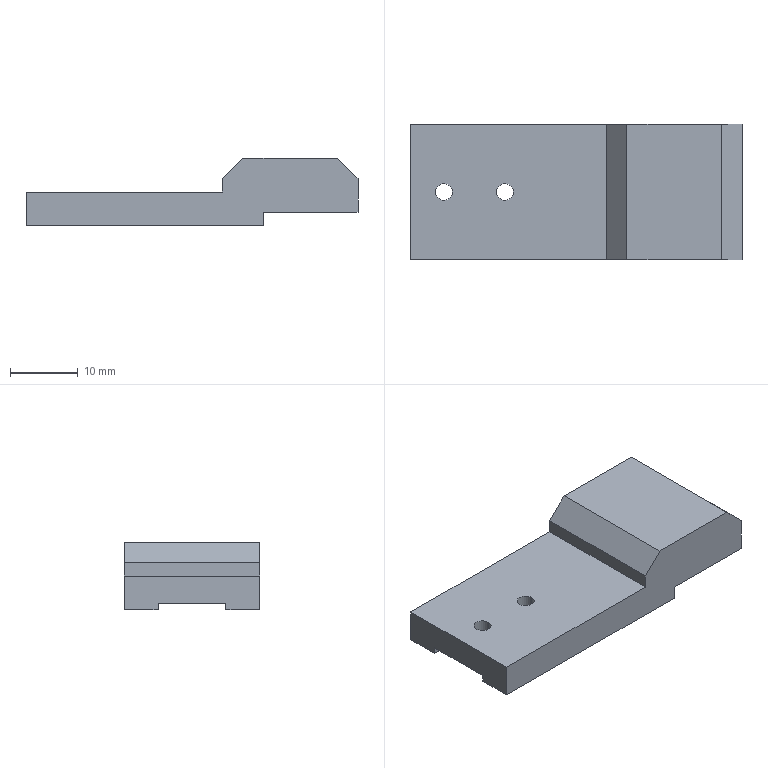Part | SolidWorks | features ICE 4, Chamfer 2, Extrusion 1, HoleWzd 1, MoveFace 1 | 1 solid | 20 faces | box 49 x 20 x 10 mm | volume 5771 mm3 | plane 16 | cylinder 4 | commonest cylinder face diameters 2.5 x4
STEP:
#1=CARTESIAN_POINT('',(-8.75,0.,1.));
#2=VERTEX_POINT('',#1);
#3=CARTESIAN_POINT('',(-11.25,0.,1.));
#4=VERTEX_POINT('',#3);
#5=CARTESIAN_POINT('',(-10.,0.,1.));
#6=DIRECTION('',(0.,0.,-1.));
#7=DIRECTION('',(-1.,0.,0.));
#8=AXIS2_PLACEMENT_3D('',#5,#6,#7);
#9=CIRCLE('',#8,1.25);
#10=EDGE_CURVE('',#2,#4,#9,.T.);
#11=ORIENTED_EDGE('',*,*,#10,.T.);
#12=CARTESIAN_POINT('',(-11.25,0.,5.));
#13=VERTEX_POINT('',#12);
#14=CARTESIAN_POINT('',(-11.25,0.,5.));
#15=DIRECTION('',(0.,0.,1.));
#16=VECTOR('',#15,1000.);
#17=LINE('',#14,#16);
#18=EDGE_CURVE('',#4,#13,#17,.T.);
#19=ORIENTED_EDGE('',*,*,#18,.T.);
#20=CARTESIAN_POINT('',(-8.75,0.,5.));
#21=VERTEX_POINT('',#20);
#22=CARTESIAN_POINT('',(-10.,0.,5.));
#23=DIRECTION('',(0.,0.,1.));
#24=DIRECTION('',(1.,0.,0.));
#25=AXIS2_PLACEMENT_3D('',#22,#23,#24);
#26=CIRCLE('',#25,1.25);
#27=EDGE_CURVE('',#13,#21,#26,.T.);
#28=ORIENTED_EDGE('',*,*,#27,.T.);
#29=CARTESIAN_POINT('',(-8.75,0.,5.));
#30=DIRECTION('',(0.,0.,1.));
#31=VECTOR('',#30,1000.);
#32=LINE('',#29,#31);
#33=EDGE_CURVE('',#2,#21,#32,.T.);
#34=ORIENTED_EDGE('',*,*,#33,.F.);
#35=EDGE_LOOP('',(#11,#19,#28,#34));
#36=FACE_OUTER_BOUND('',#35,.T.);
#37=CARTESIAN_POINT('',(-10.,0.,5.));
#38=DIRECTION('',(0.,0.,1.));
#39=DIRECTION('',(1.,0.,0.));
#40=AXIS2_PLACEMENT_3D('',#37,#38,#39);
#41=CYLINDRICAL_SURFACE('',#40,1.25);
#42=ADVANCED_FACE('',(#36),#41,.F.);
#43=CARTESIAN_POINT('',(0.25,0.,1.));
#44=VERTEX_POINT('',#43);
#45=CARTESIAN_POINT('',(-2.25,0.,1.));
#46=VERTEX_POINT('',#45);
#47=CARTESIAN_POINT('',(-1.,0.,1.));
#48=DIRECTION('',(0.,0.,-1.));
#49=DIRECTION('',(-1.,0.,0.));
#50=AXIS2_PLACEMENT_3D('',#47,#48,#49);
#51=CIRCLE('',#50,1.25);
#52=EDGE_CURVE('',#44,#46,#51,.T.);
#53=ORIENTED_EDGE('',*,*,#52,.T.);
#54=CARTESIAN_POINT('',(-2.25,0.,5.));
#55=VERTEX_POINT('',#54);
#56=CARTESIAN_POINT('',(-2.25,0.,5.));
#57=DIRECTION('',(0.,0.,1.));
#58=VECTOR('',#57,1000.);
#59=LINE('',#56,#58);
#60=EDGE_CURVE('',#46,#55,#59,.T.);
#61=ORIENTED_EDGE('',*,*,#60,.T.);
#62=CARTESIAN_POINT('',(0.25,0.,5.));
#63=VERTEX_POINT('',#62);
#64=CARTESIAN_POINT('',(-1.,0.,5.));
#65=DIRECTION('',(0.,0.,1.));
#66=DIRECTION('',(1.,0.,0.));
#67=AXIS2_PLACEMENT_3D('',#64,#65,#66);
#68=CIRCLE('',#67,1.25);
#69=EDGE_CURVE('',#55,#63,#68,.T.);
#70=ORIENTED_EDGE('',*,*,#69,.T.);
#71=CARTESIAN_POINT('',(0.25,0.,5.));
#72=DIRECTION('',(0.,0.,1.));
#73=VECTOR('',#72,1000.);
#74=LINE('',#71,#73);
#75=EDGE_CURVE('',#44,#63,#74,.T.);
#76=ORIENTED_EDGE('',*,*,#75,.F.);
#77=EDGE_LOOP('',(#53,#61,#70,#76));
#78=FACE_OUTER_BOUND('',#77,.T.);
#79=CARTESIAN_POINT('',(-1.,0.,5.));
#80=DIRECTION('',(0.,0.,1.));
#81=DIRECTION('',(1.,0.,0.));
#82=AXIS2_PLACEMENT_3D('',#79,#80,#81);
#83=CYLINDRICAL_SURFACE('',#82,1.25);
#84=ADVANCED_FACE('',(#78),#83,.F.);
#85=CARTESIAN_POINT('',(-15.,-5.,0.));
#86=VERTEX_POINT('',#85);
#87=CARTESIAN_POINT('',(-15.,-10.,0.));
#88=VERTEX_POINT('',#87);
#89=CARTESIAN_POINT('',(-15.,10.,0.));
#90=DIRECTION('',(0.,-1.,0.));
#91=VECTOR('',#90,1000.);
#92=LINE('',#89,#91);
#93=EDGE_CURVE('',#86,#88,#92,.T.);
#94=ORIENTED_EDGE('',*,*,#93,.F.);
#95=CARTESIAN_POINT('',(20.,-5.,0.));
#96=VERTEX_POINT('',#95);
#97=CARTESIAN_POINT('',(-15.,-5.,0.));
#98=DIRECTION('',(-1.,0.,0.));
#99=VECTOR('',#98,1000.);
#100=LINE('',#97,#99);
#101=EDGE_CURVE('',#96,#86,#100,.T.);
#102=ORIENTED_EDGE('',*,*,#101,.F.);
#103=CARTESIAN_POINT('',(20.,-10.,0.));
#104=VERTEX_POINT('',#103);
#105=CARTESIAN_POINT('',(20.,10.,0.));
#106=DIRECTION('',(0.,1.,0.));
#107=VECTOR('',#106,1000.);
#108=LINE('',#105,#107);
#109=EDGE_CURVE('',#104,#96,#108,.T.);
#110=ORIENTED_EDGE('',*,*,#109,.F.);
#111=CARTESIAN_POINT('',(-15.,-10.,0.));
#112=DIRECTION('',(1.,0.,0.));
#113=VECTOR('',#112,1000.);
#114=LINE('',#111,#113);
#115=EDGE_CURVE('',#88,#104,#114,.T.);
#116=ORIENTED_EDGE('',*,*,#115,.F.);
#117=EDGE_LOOP('',(#94,#102,#110,#116));
#118=FACE_OUTER_BOUND('',#117,.T.);
#119=CARTESIAN_POINT('',(0.,0.,0.));
#120=DIRECTION('',(0.,0.,1.));
#121=DIRECTION('',(1.,0.,0.));
#122=AXIS2_PLACEMENT_3D('',#119,#120,#121);
#123=PLANE('',#122);
#124=ADVANCED_FACE('',(#118),#123,.F.);
#125=CARTESIAN_POINT('',(31.,10.,10.));
#126=VERTEX_POINT('',#125);
#127=CARTESIAN_POINT('',(17.,10.,10.));
#128=VERTEX_POINT('',#127);
#129=CARTESIAN_POINT('',(14.,10.,10.));
#130=DIRECTION('',(-1.,0.,0.));
#131=VECTOR('',#130,1000.);
#132=LINE('',#129,#131);
#133=EDGE_CURVE('',#126,#128,#132,.T.);
#134=ORIENTED_EDGE('',*,*,#133,.F.);
#135=CARTESIAN_POINT('',(34.,10.,7.));
#136=VERTEX_POINT('',#135);
#137=CARTESIAN_POINT('',(31.,10.,10.));
#138=DIRECTION('',(0.7071,0.,-0.7071));
#139=VECTOR('',#138,1000.);
#140=LINE('',#137,#139);
#141=EDGE_CURVE('',#126,#136,#140,.T.);
#142=ORIENTED_EDGE('',*,*,#141,.T.);
#143=CARTESIAN_POINT('',(34.,10.,2.));
#144=VERTEX_POINT('',#143);
#145=CARTESIAN_POINT('',(34.,10.,10.));
#146=DIRECTION('',(0.,0.,-1.));
#147=VECTOR('',#146,1000.);
#148=LINE('',#145,#147);
#149=EDGE_CURVE('',#136,#144,#148,.T.);
#150=ORIENTED_EDGE('',*,*,#149,.T.);
#151=CARTESIAN_POINT('',(20.,10.,2.));
#152=VERTEX_POINT('',#151);
#153=CARTESIAN_POINT('',(14.,10.,2.));
#154=DIRECTION('',(-1.,0.,0.));
#155=VECTOR('',#154,1000.);
#156=LINE('',#153,#155);
#157=EDGE_CURVE('',#144,#152,#156,.T.);
#158=ORIENTED_EDGE('',*,*,#157,.T.);
#159=CARTESIAN_POINT('',(20.,10.,0.));
#160=VERTEX_POINT('',#159);
#161=CARTESIAN_POINT('',(20.,10.,0.));
#162=DIRECTION('',(0.,0.,1.));
#163=VECTOR('',#162,1000.);
#164=LINE('',#161,#163);
#165=EDGE_CURVE('',#160,#152,#164,.T.);
#166=ORIENTED_EDGE('',*,*,#165,.F.);
#167=CARTESIAN_POINT('',(-15.,10.,0.));
#168=VERTEX_POINT('',#167);
#169=CARTESIAN_POINT('',(-15.,10.,0.));
#170=DIRECTION('',(-1.,0.,0.));
#171=VECTOR('',#170,1000.);
#172=LINE('',#169,#171);
#173=EDGE_CURVE('',#160,#168,#172,.T.);
#174=ORIENTED_EDGE('',*,*,#173,.T.);
#175=CARTESIAN_POINT('',(-15.,10.,5.));
#176=VERTEX_POINT('',#175);
#177=CARTESIAN_POINT('',(-15.,10.,5.));
#178=DIRECTION('',(0.,0.,-1.));
#179=VECTOR('',#178,1000.);
#180=LINE('',#177,#179);
#181=EDGE_CURVE('',#176,#168,#180,.T.);
#182=ORIENTED_EDGE('',*,*,#181,.F.);
#183=CARTESIAN_POINT('',(14.,10.,5.));
#184=VERTEX_POINT('',#183);
#185=CARTESIAN_POINT('',(-15.,10.,5.));
#186=DIRECTION('',(-1.,0.,0.));
#187=VECTOR('',#186,1000.);
#188=LINE('',#185,#187);
#189=EDGE_CURVE('',#184,#176,#188,.T.);
#190=ORIENTED_EDGE('',*,*,#189,.F.);
#191=CARTESIAN_POINT('',(14.,10.,7.));
#192=VERTEX_POINT('',#191);
#193=CARTESIAN_POINT('',(14.,10.,10.));
#194=DIRECTION('',(0.,0.,-1.));
#195=VECTOR('',#194,1000.);
#196=LINE('',#193,#195);
#197=EDGE_CURVE('',#192,#184,#196,.T.);
#198=ORIENTED_EDGE('',*,*,#197,.F.);
#199=CARTESIAN_POINT('',(17.,10.,10.));
#200=DIRECTION('',(0.7071,0.,0.7071));
#201=VECTOR('',#200,1000.);
#202=LINE('',#199,#201);
#203=EDGE_CURVE('',#192,#128,#202,.T.);
#204=ORIENTED_EDGE('',*,*,#203,.T.);
#205=EDGE_LOOP('',(#134,#142,#150,#158,#166,#174,#182,#190,#198,#204));
#206=FACE_OUTER_BOUND('',#205,.T.);
#207=CARTESIAN_POINT('',(-15.,10.,5.));
#208=DIRECTION('',(0.,-1.,0.));
#209=DIRECTION('',(0.,0.,-1.));
#210=AXIS2_PLACEMENT_3D('',#207,#208,#209);
#211=PLANE('',#210);
#212=ADVANCED_FACE('',(#206),#211,.F.);
#213=CARTESIAN_POINT('',(-15.,-5.,1.));
#214=VERTEX_POINT('',#213);
#215=CARTESIAN_POINT('',(-15.,5.,1.));
#216=VERTEX_POINT('',#215);
#217=CARTESIAN_POINT('',(-15.,-5.,1.));
#218=DIRECTION('',(0.,1.,0.));
#219=VECTOR('',#218,1000.);
#220=LINE('',#217,#219);
#221=EDGE_CURVE('',#214,#216,#220,.T.);
#222=ORIENTED_EDGE('',*,*,#221,.F.);
#223=CARTESIAN_POINT('',(-15.,-5.,1.));
#224=DIRECTION('',(0.,0.,-1.));
#225=VECTOR('',#224,1000.);
#226=LINE('',#223,#225);
#227=EDGE_CURVE('',#214,#86,#226,.T.);
#228=ORIENTED_EDGE('',*,*,#227,.T.);
#229=ORIENTED_EDGE('',*,*,#93,.T.);
#230=CARTESIAN_POINT('',(-15.,-10.,5.));
#231=VERTEX_POINT('',#230);
#232=CARTESIAN_POINT('',(-15.,-10.,5.));
#233=DIRECTION('',(0.,0.,-1.));
#234=VECTOR('',#233,1000.);
#235=LINE('',#232,#234);
#236=EDGE_CURVE('',#231,#88,#235,.T.);
#237=ORIENTED_EDGE('',*,*,#236,.F.);
#238=CARTESIAN_POINT('',(-15.,10.,5.));
#239=DIRECTION('',(0.,-1.,0.));
#240=VECTOR('',#239,1000.);
#241=LINE('',#238,#240);
#242=EDGE_CURVE('',#176,#231,#241,.T.);
#243=ORIENTED_EDGE('',*,*,#242,.F.);
#244=ORIENTED_EDGE('',*,*,#181,.T.);
#245=CARTESIAN_POINT('',(-15.,5.,0.));
#246=VERTEX_POINT('',#245);
#247=CARTESIAN_POINT('',(-15.,10.,0.));
#248=DIRECTION('',(0.,-1.,0.));
#249=VECTOR('',#248,1000.);
#250=LINE('',#247,#249);
#251=EDGE_CURVE('',#168,#246,#250,.T.);
#252=ORIENTED_EDGE('',*,*,#251,.T.);
#253=CARTESIAN_POINT('',(-15.,5.,1.));
#254=DIRECTION('',(0.,0.,-1.));
#255=VECTOR('',#254,1000.);
#256=LINE('',#253,#255);
#257=EDGE_CURVE('',#216,#246,#256,.T.);
#258=ORIENTED_EDGE('',*,*,#257,.F.);
#259=EDGE_LOOP('',(#222,#228,#229,#237,#243,#244,#252,#258));
#260=FACE_OUTER_BOUND('',#259,.T.);
#261=CARTESIAN_POINT('',(-15.,10.,5.));
#262=DIRECTION('',(1.,0.,0.));
#263=DIRECTION('',(0.,1.,0.));
#264=AXIS2_PLACEMENT_3D('',#261,#262,#263);
#265=PLANE('',#264);
#266=ADVANCED_FACE('',(#260),#265,.F.);
#267=CARTESIAN_POINT('',(34.,-10.,7.));
#268=VERTEX_POINT('',#267);
#269=CARTESIAN_POINT('',(34.,-10.,2.));
#270=VERTEX_POINT('',#269);
#271=CARTESIAN_POINT('',(34.,-10.,10.));
#272=DIRECTION('',(0.,0.,-1.));
#273=VECTOR('',#272,1000.);
#274=LINE('',#271,#273);
#275=EDGE_CURVE('',#268,#270,#274,.T.);
#276=ORIENTED_EDGE('',*,*,#275,.F.);
#277=CARTESIAN_POINT('',(31.,-10.,10.));
#278=VERTEX_POINT('',#277);
#279=CARTESIAN_POINT('',(31.,-10.,10.));
#280=DIRECTION('',(-0.7071,0.,0.7071));
#281=VECTOR('',#280,1000.);
#282=LINE('',#279,#281);
#283=EDGE_CURVE('',#268,#278,#282,.T.);
#284=ORIENTED_EDGE('',*,*,#283,.T.);
#285=CARTESIAN_POINT('',(17.,-10.,10.));
#286=VERTEX_POINT('',#285);
#287=CARTESIAN_POINT('',(14.,-10.,10.));
#288=DIRECTION('',(1.,0.,0.));
#289=VECTOR('',#288,1000.);
#290=LINE('',#287,#289);
#291=EDGE_CURVE('',#286,#278,#290,.T.);
#292=ORIENTED_EDGE('',*,*,#291,.F.);
#293=CARTESIAN_POINT('',(14.,-10.,7.));
#294=VERTEX_POINT('',#293);
#295=CARTESIAN_POINT('',(17.,-10.,10.));
#296=DIRECTION('',(-0.7071,0.,-0.7071));
#297=VECTOR('',#296,1000.);
#298=LINE('',#295,#297);
#299=EDGE_CURVE('',#286,#294,#298,.T.);
#300=ORIENTED_EDGE('',*,*,#299,.T.);
#301=CARTESIAN_POINT('',(14.,-10.,5.));
#302=VERTEX_POINT('',#301);
#303=CARTESIAN_POINT('',(14.,-10.,10.));
#304=DIRECTION('',(0.,0.,-1.));
#305=VECTOR('',#304,1000.);
#306=LINE('',#303,#305);
#307=EDGE_CURVE('',#294,#302,#306,.T.);
#308=ORIENTED_EDGE('',*,*,#307,.T.);
#309=CARTESIAN_POINT('',(-15.,-10.,5.));
#310=DIRECTION('',(1.,0.,0.));
#311=VECTOR('',#310,1000.);
#312=LINE('',#309,#311);
#313=EDGE_CURVE('',#231,#302,#312,.T.);
#314=ORIENTED_EDGE('',*,*,#313,.F.);
#315=ORIENTED_EDGE('',*,*,#236,.T.);
#316=ORIENTED_EDGE('',*,*,#115,.T.);
#317=CARTESIAN_POINT('',(20.,-10.,2.));
#318=VERTEX_POINT('',#317);
#319=CARTESIAN_POINT('',(20.,-10.,0.));
#320=DIRECTION('',(0.,0.,-1.));
#321=VECTOR('',#320,1000.);
#322=LINE('',#319,#321);
#323=EDGE_CURVE('',#318,#104,#322,.T.);
#324=ORIENTED_EDGE('',*,*,#323,.F.);
#325=CARTESIAN_POINT('',(14.,-10.,2.));
#326=DIRECTION('',(1.,0.,0.));
#327=VECTOR('',#326,1000.);
#328=LINE('',#325,#327);
#329=EDGE_CURVE('',#318,#270,#328,.T.);
#330=ORIENTED_EDGE('',*,*,#329,.T.);
#331=EDGE_LOOP('',(#276,#284,#292,#300,#308,#314,#315,#316,#324,#330));
#332=FACE_OUTER_BOUND('',#331,.T.);
#333=CARTESIAN_POINT('',(-15.,-10.,5.));
#334=DIRECTION('',(0.,1.,0.));
#335=DIRECTION('',(0.,0.,1.));
#336=AXIS2_PLACEMENT_3D('',#333,#334,#335);
#337=PLANE('',#336);
#338=ADVANCED_FACE('',(#332),#337,.F.);
#339=CARTESIAN_POINT('',(-10.,0.,5.));
#340=DIRECTION('',(0.,0.,1.));
#341=DIRECTION('',(1.,0.,0.));
#342=AXIS2_PLACEMENT_3D('',#339,#340,#341);
#343=CIRCLE('',#342,1.25);
#344=EDGE_CURVE('',#21,#13,#343,.T.);
#345=ORIENTED_EDGE('',*,*,#344,.F.);
#346=ORIENTED_EDGE('',*,*,#27,.F.);
#347=EDGE_LOOP('',(#345,#346));
#348=FACE_BOUND('',#347,.T.);
#349=CARTESIAN_POINT('',(-1.,0.,5.));
#350=DIRECTION('',(0.,0.,1.));
#351=DIRECTION('',(1.,0.,0.));
#352=AXIS2_PLACEMENT_3D('',#349,#350,#351);
#353=CIRCLE('',#352,1.25);
#354=EDGE_CURVE('',#63,#55,#353,.T.);
#355=ORIENTED_EDGE('',*,*,#354,.F.);
#356=ORIENTED_EDGE('',*,*,#69,.F.);
#357=EDGE_LOOP('',(#355,#356));
#358=FACE_BOUND('',#357,.T.);
#359=CARTESIAN_POINT('',(14.,10.,5.));
#360=DIRECTION('',(0.,-1.,0.));
#361=VECTOR('',#360,1000.);
#362=LINE('',#359,#361);
#363=EDGE_CURVE('',#184,#302,#362,.T.);
#364=ORIENTED_EDGE('',*,*,#363,.F.);
#365=ORIENTED_EDGE('',*,*,#189,.T.);
#366=ORIENTED_EDGE('',*,*,#242,.T.);
#367=ORIENTED_EDGE('',*,*,#313,.T.);
#368=EDGE_LOOP('',(#364,#365,#366,#367));
#369=FACE_OUTER_BOUND('',#368,.T.);
#370=CARTESIAN_POINT('',(0.,0.,5.));
#371=DIRECTION('',(0.,0.,1.));
#372=DIRECTION('',(1.,0.,0.));
#373=AXIS2_PLACEMENT_3D('',#370,#371,#372);
#374=PLANE('',#373);
#375=ADVANCED_FACE('',(#348,#358,#369),#374,.T.);
#376=CARTESIAN_POINT('',(20.,5.,0.));
#377=VERTEX_POINT('',#376);
#378=CARTESIAN_POINT('',(20.,10.,0.));
#379=DIRECTION('',(0.,1.,0.));
#380=VECTOR('',#379,1000.);
#381=LINE('',#378,#380);
#382=EDGE_CURVE('',#377,#160,#381,.T.);
#383=ORIENTED_EDGE('',*,*,#382,.F.);
#384=CARTESIAN_POINT('',(-15.,5.,0.));
#385=DIRECTION('',(1.,0.,0.));
#386=VECTOR('',#385,1000.);
#387=LINE('',#384,#386);
#388=EDGE_CURVE('',#246,#377,#387,.T.);
#389=ORIENTED_EDGE('',*,*,#388,.F.);
#390=ORIENTED_EDGE('',*,*,#251,.F.);
#391=ORIENTED_EDGE('',*,*,#173,.F.);
#392=EDGE_LOOP('',(#383,#389,#390,#391));
#393=FACE_OUTER_BOUND('',#392,.T.);
#394=CARTESIAN_POINT('',(0.,0.,0.));
#395=DIRECTION('',(0.,0.,1.));
#396=DIRECTION('',(1.,0.,0.));
#397=AXIS2_PLACEMENT_3D('',#394,#395,#396);
#398=PLANE('',#397);
#399=ADVANCED_FACE('',(#393),#398,.F.);
#400=ORIENTED_EDGE('',*,*,#109,.T.);
#401=CARTESIAN_POINT('',(20.,-5.,1.));
#402=VERTEX_POINT('',#401);
#403=CARTESIAN_POINT('',(20.,-5.,1.));
#404=DIRECTION('',(0.,0.,-1.));
#405=VECTOR('',#404,1000.);
#406=LINE('',#403,#405);
#407=EDGE_CURVE('',#402,#96,#406,.T.);
#408=ORIENTED_EDGE('',*,*,#407,.F.);
#409=CARTESIAN_POINT('',(20.,5.,1.));
#410=VERTEX_POINT('',#409);
#411=CARTESIAN_POINT('',(20.,-5.,1.));
#412=DIRECTION('',(0.,-1.,0.));
#413=VECTOR('',#412,1000.);
#414=LINE('',#411,#413);
#415=EDGE_CURVE('',#410,#402,#414,.T.);
#416=ORIENTED_EDGE('',*,*,#415,.F.);
#417=CARTESIAN_POINT('',(20.,5.,1.));
#418=DIRECTION('',(0.,0.,-1.));
#419=VECTOR('',#418,1000.);
#420=LINE('',#417,#419);
#421=EDGE_CURVE('',#410,#377,#420,.T.);
#422=ORIENTED_EDGE('',*,*,#421,.T.);
#423=ORIENTED_EDGE('',*,*,#382,.T.);
#424=ORIENTED_EDGE('',*,*,#165,.T.);
#425=CARTESIAN_POINT('',(20.,10.,2.));
#426=DIRECTION('',(0.,-1.,0.));
#427=VECTOR('',#426,1000.);
#428=LINE('',#425,#427);
#429=EDGE_CURVE('',#152,#318,#428,.T.);
#430=ORIENTED_EDGE('',*,*,#429,.T.);
#431=ORIENTED_EDGE('',*,*,#323,.T.);
#432=EDGE_LOOP('',(#400,#408,#416,#422,#423,#424,#430,#431));
#433=FACE_OUTER_BOUND('',#432,.T.);
#434=CARTESIAN_POINT('',(20.,0.,0.));
#435=DIRECTION('',(-1.,0.,0.));
#436=DIRECTION('',(0.,0.,1.));
#437=AXIS2_PLACEMENT_3D('',#434,#435,#436);
#438=PLANE('',#437);
#439=ADVANCED_FACE('',(#433),#438,.F.);
#440=ORIENTED_EDGE('',*,*,#101,.T.);
#441=ORIENTED_EDGE('',*,*,#227,.F.);
#442=CARTESIAN_POINT('',(-15.,-5.,1.));
#443=DIRECTION('',(-1.,0.,0.));
#444=VECTOR('',#443,1000.);
#445=LINE('',#442,#444);
#446=EDGE_CURVE('',#402,#214,#445,.T.);
#447=ORIENTED_EDGE('',*,*,#446,.F.);
#448=ORIENTED_EDGE('',*,*,#407,.T.);
#449=EDGE_LOOP('',(#440,#441,#447,#448));
#450=FACE_OUTER_BOUND('',#449,.T.);
#451=CARTESIAN_POINT('',(-15.,-5.,1.));
#452=DIRECTION('',(0.,-1.,0.));
#453=DIRECTION('',(1.,0.,0.));
#454=AXIS2_PLACEMENT_3D('',#451,#452,#453);
#455=PLANE('',#454);
#456=ADVANCED_FACE('',(#450),#455,.F.);
#457=ORIENTED_EDGE('',*,*,#388,.T.);
#458=ORIENTED_EDGE('',*,*,#421,.F.);
#459=CARTESIAN_POINT('',(-15.,5.,1.));
#460=DIRECTION('',(1.,0.,0.));
#461=VECTOR('',#460,1000.);
#462=LINE('',#459,#461);
#463=EDGE_CURVE('',#216,#410,#462,.T.);
#464=ORIENTED_EDGE('',*,*,#463,.F.);
#465=ORIENTED_EDGE('',*,*,#257,.T.);
#466=EDGE_LOOP('',(#457,#458,#464,#465));
#467=FACE_OUTER_BOUND('',#466,.T.);
#468=CARTESIAN_POINT('',(-15.,5.,1.));
#469=DIRECTION('',(0.,1.,0.));
#470=DIRECTION('',(-1.,0.,0.));
#471=AXIS2_PLACEMENT_3D('',#468,#469,#470);
#472=PLANE('',#471);
#473=ADVANCED_FACE('',(#467),#472,.F.);
#474=ORIENTED_EDGE('',*,*,#10,.F.);
#475=CARTESIAN_POINT('',(-10.,0.,1.));
#476=DIRECTION('',(0.,0.,-1.));
#477=DIRECTION('',(-1.,0.,0.));
#478=AXIS2_PLACEMENT_3D('',#475,#476,#477);
#479=CIRCLE('',#478,1.25);
#480=EDGE_CURVE('',#4,#2,#479,.T.);
#481=ORIENTED_EDGE('',*,*,#480,.F.);
#482=EDGE_LOOP('',(#474,#481));
#483=FACE_BOUND('',#482,.T.);
#484=ORIENTED_EDGE('',*,*,#52,.F.);
#485=CARTESIAN_POINT('',(-1.,0.,1.));
#486=DIRECTION('',(0.,0.,-1.));
#487=DIRECTION('',(-1.,0.,0.));
#488=AXIS2_PLACEMENT_3D('',#485,#486,#487);
#489=CIRCLE('',#488,1.25);
#490=EDGE_CURVE('',#46,#44,#489,.T.);
#491=ORIENTED_EDGE('',*,*,#490,.F.);
#492=EDGE_LOOP('',(#484,#491));
#493=FACE_BOUND('',#492,.T.);
#494=ORIENTED_EDGE('',*,*,#221,.T.);
#495=ORIENTED_EDGE('',*,*,#463,.T.);
#496=ORIENTED_EDGE('',*,*,#415,.T.);
#497=ORIENTED_EDGE('',*,*,#446,.T.);
#498=EDGE_LOOP('',(#494,#495,#496,#497));
#499=FACE_OUTER_BOUND('',#498,.T.);
#500=CARTESIAN_POINT('',(0.,0.,1.));
#501=DIRECTION('',(0.,0.,-1.));
#502=DIRECTION('',(-1.,0.,0.));
#503=AXIS2_PLACEMENT_3D('',#500,#501,#502);
#504=PLANE('',#503);
#505=ADVANCED_FACE('',(#483,#493,#499),#504,.T.);
#506=ORIENTED_EDGE('',*,*,#307,.F.);
#507=CARTESIAN_POINT('',(14.,10.,7.));
#508=DIRECTION('',(0.,1.,0.));
#509=VECTOR('',#508,1000.);
#510=LINE('',#507,#509);
#511=EDGE_CURVE('',#294,#192,#510,.T.);
#512=ORIENTED_EDGE('',*,*,#511,.T.);
#513=ORIENTED_EDGE('',*,*,#197,.T.);
#514=ORIENTED_EDGE('',*,*,#363,.T.);
#515=EDGE_LOOP('',(#506,#512,#513,#514));
#516=FACE_OUTER_BOUND('',#515,.T.);
#517=CARTESIAN_POINT('',(14.,10.,10.));
#518=DIRECTION('',(1.,0.,0.));
#519=DIRECTION('',(0.,0.,-1.));
#520=AXIS2_PLACEMENT_3D('',#517,#518,#519);
#521=PLANE('',#520);
#522=ADVANCED_FACE('',(#516),#521,.F.);
#523=ORIENTED_EDGE('',*,*,#149,.F.);
#524=CARTESIAN_POINT('',(34.,-10.,7.));
#525=DIRECTION('',(0.,-1.,0.));
#526=VECTOR('',#525,1000.);
#527=LINE('',#524,#526);
#528=EDGE_CURVE('',#136,#268,#527,.T.);
#529=ORIENTED_EDGE('',*,*,#528,.T.);
#530=ORIENTED_EDGE('',*,*,#275,.T.);
#531=CARTESIAN_POINT('',(34.,10.,2.));
#532=DIRECTION('',(0.,1.,0.));
#533=VECTOR('',#532,1000.);
#534=LINE('',#531,#533);
#535=EDGE_CURVE('',#270,#144,#534,.T.);
#536=ORIENTED_EDGE('',*,*,#535,.T.);
#537=EDGE_LOOP('',(#523,#529,#530,#536));
#538=FACE_OUTER_BOUND('',#537,.T.);
#539=CARTESIAN_POINT('',(34.,10.,10.));
#540=DIRECTION('',(-1.,0.,0.));
#541=DIRECTION('',(0.,0.,1.));
#542=AXIS2_PLACEMENT_3D('',#539,#540,#541);
#543=PLANE('',#542);
#544=ADVANCED_FACE('',(#538),#543,.F.);
#545=ORIENTED_EDGE('',*,*,#291,.T.);
#546=CARTESIAN_POINT('',(31.,10.,10.));
#547=DIRECTION('',(0.,1.,0.));
#548=VECTOR('',#547,1000.);
#549=LINE('',#546,#548);
#550=EDGE_CURVE('',#278,#126,#549,.T.);
#551=ORIENTED_EDGE('',*,*,#550,.T.);
#552=ORIENTED_EDGE('',*,*,#133,.T.);
#553=CARTESIAN_POINT('',(17.,-10.,10.));
#554=DIRECTION('',(0.,-1.,0.));
#555=VECTOR('',#554,1000.);
#556=LINE('',#553,#555);
#557=EDGE_CURVE('',#128,#286,#556,.T.);
#558=ORIENTED_EDGE('',*,*,#557,.T.);
#559=EDGE_LOOP('',(#545,#551,#552,#558));
#560=FACE_OUTER_BOUND('',#559,.T.);
#561=CARTESIAN_POINT('',(0.,0.,10.));
#562=DIRECTION('',(0.,0.,1.));
#563=DIRECTION('',(1.,0.,0.));
#564=AXIS2_PLACEMENT_3D('',#561,#562,#563);
#565=PLANE('',#564);
#566=ADVANCED_FACE('',(#560),#565,.T.);
#567=ORIENTED_EDGE('',*,*,#429,.F.);
#568=ORIENTED_EDGE('',*,*,#157,.F.);
#569=ORIENTED_EDGE('',*,*,#535,.F.);
#570=ORIENTED_EDGE('',*,*,#329,.F.);
#571=EDGE_LOOP('',(#567,#568,#569,#570));
#572=FACE_OUTER_BOUND('',#571,.T.);
#573=CARTESIAN_POINT('',(0.,0.,2.));
#574=DIRECTION('',(0.,0.,1.));
#575=DIRECTION('',(1.,0.,0.));
#576=AXIS2_PLACEMENT_3D('',#573,#574,#575);
#577=PLANE('',#576);
#578=ADVANCED_FACE('',(#572),#577,.F.);
#579=ORIENTED_EDGE('',*,*,#203,.F.);
#580=ORIENTED_EDGE('',*,*,#511,.F.);
#581=ORIENTED_EDGE('',*,*,#299,.F.);
#582=ORIENTED_EDGE('',*,*,#557,.F.);
#583=EDGE_LOOP('',(#579,#580,#581,#582));
#584=FACE_OUTER_BOUND('',#583,.T.);
#585=CARTESIAN_POINT('',(17.,0.,10.));
#586=DIRECTION('',(-0.7071,0.,0.7071));
#587=DIRECTION('',(0.,1.,0.));
#588=AXIS2_PLACEMENT_3D('',#585,#586,#587);
#589=PLANE('',#588);
#590=ADVANCED_FACE('',(#584),#589,.T.);
#591=ORIENTED_EDGE('',*,*,#283,.F.);
#592=ORIENTED_EDGE('',*,*,#528,.F.);
#593=ORIENTED_EDGE('',*,*,#141,.F.);
#594=ORIENTED_EDGE('',*,*,#550,.F.);
#595=EDGE_LOOP('',(#591,#592,#593,#594));
#596=FACE_OUTER_BOUND('',#595,.T.);
#597=CARTESIAN_POINT('',(31.,0.,10.));
#598=DIRECTION('',(0.7071,0.,0.7071));
#599=DIRECTION('',(0.,-1.,0.));
#600=AXIS2_PLACEMENT_3D('',#597,#598,#599);
#601=PLANE('',#600);
#602=ADVANCED_FACE('',(#596),#601,.T.);
#603=ORIENTED_EDGE('',*,*,#60,.F.);
#604=ORIENTED_EDGE('',*,*,#490,.T.);
#605=ORIENTED_EDGE('',*,*,#75,.T.);
#606=ORIENTED_EDGE('',*,*,#354,.T.);
#607=EDGE_LOOP('',(#603,#604,#605,#606));
#608=FACE_OUTER_BOUND('',#607,.T.);
#609=CARTESIAN_POINT('',(-1.,0.,5.));
#610=DIRECTION('',(0.,0.,1.));
#611=DIRECTION('',(1.,0.,0.));
#612=AXIS2_PLACEMENT_3D('',#609,#610,#611);
#613=CYLINDRICAL_SURFACE('',#612,1.25);
#614=ADVANCED_FACE('',(#608),#613,.F.);
#615=ORIENTED_EDGE('',*,*,#18,.F.);
#616=ORIENTED_EDGE('',*,*,#480,.T.);
#617=ORIENTED_EDGE('',*,*,#33,.T.);
#618=ORIENTED_EDGE('',*,*,#344,.T.);
#619=EDGE_LOOP('',(#615,#616,#617,#618));
#620=FACE_OUTER_BOUND('',#619,.T.);
#621=CARTESIAN_POINT('',(-10.,0.,5.));
#622=DIRECTION('',(0.,0.,1.));
#623=DIRECTION('',(1.,0.,0.));
#624=AXIS2_PLACEMENT_3D('',#621,#622,#623);
#625=CYLINDRICAL_SURFACE('',#624,1.25);
#626=ADVANCED_FACE('',(#620),#625,.F.);
#627=CLOSED_SHELL('',(#42,#84,#124,#212,#266,#338,#375,#399,#439,#456,#473,#505,#522,#544,#566,#578,#590,#602,#614,#626));
#628=MANIFOLD_SOLID_BREP('',#627);
#629=CARTESIAN_POINT('',(0.,0.,0.));
#630=DIRECTION('',(0.,0.,1.));
#631=DIRECTION('',(1.,0.,0.));
#632=AXIS2_PLACEMENT_3D('',#629,#630,#631);
#633=(LENGTH_UNIT()NAMED_UNIT(*)SI_UNIT(.MILLI.,.METRE.));
#634=UNCERTAINTY_MEASURE_WITH_UNIT(LENGTH_MEASURE(0.00001),#633,'','');
#635=(NAMED_UNIT(*)PLANE_ANGLE_UNIT()SI_UNIT($,.RADIAN.));
#636=(NAMED_UNIT(*)SI_UNIT($,.STERADIAN.)SOLID_ANGLE_UNIT());
#637=(GEOMETRIC_REPRESENTATION_CONTEXT(3)GLOBAL_UNCERTAINTY_ASSIGNED_CONTEXT((#634))GLOBAL_UNIT_ASSIGNED_CONTEXT((#633,#635,#636))REPRESENTATION_CONTEXT('',''));
#638=ADVANCED_BREP_SHAPE_REPRESENTATION('',(#628,#632),#637);